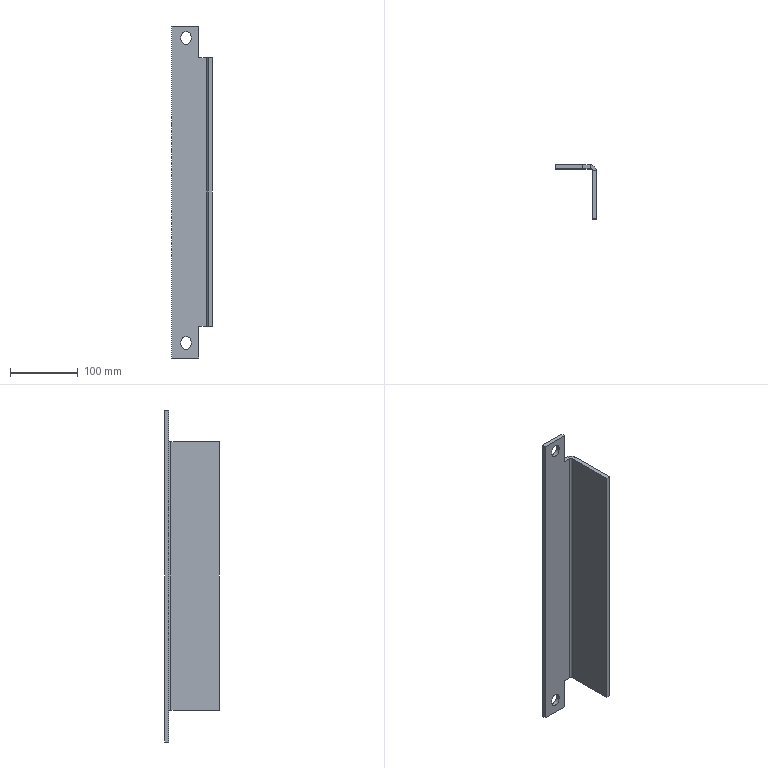Part | SolidWorks | features ICE 2, FlatPattern 1, SMBaseFlange 1, SheetMetal 1 | 1 solid | 28 faces | box 60 x 80 x 490 mm | volume 331985 mm3 | plane 20 | cylinder 8 | commonest cylinder face diameters 15 x6 6 x1 18 x1
STEP:
#1=CARTESIAN_POINT('',(-38.8,-6.,-213.5));
#2=VERTEX_POINT('',#1);
#3=CARTESIAN_POINT('',(-31.3,-6.,-221.));
#4=VERTEX_POINT('',#3);
#5=CARTESIAN_POINT('',(-38.8,-6.,-221.));
#6=DIRECTION('',(0.,1.,0.));
#7=DIRECTION('',(-1.,0.,0.));
#8=AXIS2_PLACEMENT_3D('',#5,#6,#7);
#9=CIRCLE('',#8,7.5);
#10=EDGE_CURVE('',#2,#4,#9,.T.);
#11=ORIENTED_EDGE('',*,*,#10,.F.);
#12=CARTESIAN_POINT('',(-38.8,0.,-213.5));
#13=VERTEX_POINT('',#12);
#14=CARTESIAN_POINT('',(-38.8,-80.,-213.5));
#15=DIRECTION('',(0.,1.,0.));
#16=VECTOR('',#15,1000.);
#17=LINE('',#14,#16);
#18=EDGE_CURVE('',#2,#13,#17,.T.);
#19=ORIENTED_EDGE('',*,*,#18,.T.);
#20=CARTESIAN_POINT('',(-31.3,0.,-221.));
#21=VERTEX_POINT('',#20);
#22=CARTESIAN_POINT('',(-38.8,0.,-221.));
#23=DIRECTION('',(0.,1.,0.));
#24=DIRECTION('',(0.,0.,1.));
#25=AXIS2_PLACEMENT_3D('',#22,#23,#24);
#26=CIRCLE('',#25,7.5);
#27=EDGE_CURVE('',#13,#21,#26,.T.);
#28=ORIENTED_EDGE('',*,*,#27,.T.);
#29=CARTESIAN_POINT('',(-31.3,-80.,-221.));
#30=DIRECTION('',(0.,1.,0.));
#31=VECTOR('',#30,1000.);
#32=LINE('',#29,#31);
#33=EDGE_CURVE('',#4,#21,#32,.T.);
#34=ORIENTED_EDGE('',*,*,#33,.F.);
#35=EDGE_LOOP('',(#11,#19,#28,#34));
#36=FACE_OUTER_BOUND('',#35,.T.);
#37=CARTESIAN_POINT('',(-38.8,-80.,-221.));
#38=DIRECTION('',(0.,1.,0.));
#39=DIRECTION('',(0.,0.,1.));
#40=AXIS2_PLACEMENT_3D('',#37,#38,#39);
#41=CYLINDRICAL_SURFACE('',#40,7.5);
#42=ADVANCED_FACE('',(#36),#41,.F.);
#43=CARTESIAN_POINT('',(-38.8,-6.,236.5));
#44=VERTEX_POINT('',#43);
#45=CARTESIAN_POINT('',(-31.3,-6.,229.));
#46=VERTEX_POINT('',#45);
#47=CARTESIAN_POINT('',(-38.8,-6.,229.));
#48=DIRECTION('',(0.,1.,0.));
#49=DIRECTION('',(-1.,0.,0.));
#50=AXIS2_PLACEMENT_3D('',#47,#48,#49);
#51=CIRCLE('',#50,7.5);
#52=EDGE_CURVE('',#44,#46,#51,.T.);
#53=ORIENTED_EDGE('',*,*,#52,.F.);
#54=CARTESIAN_POINT('',(-38.8,0.,236.5));
#55=VERTEX_POINT('',#54);
#56=CARTESIAN_POINT('',(-38.8,-80.,236.5));
#57=DIRECTION('',(0.,1.,0.));
#58=VECTOR('',#57,1000.);
#59=LINE('',#56,#58);
#60=EDGE_CURVE('',#44,#55,#59,.T.);
#61=ORIENTED_EDGE('',*,*,#60,.T.);
#62=CARTESIAN_POINT('',(-31.3,0.,229.));
#63=VERTEX_POINT('',#62);
#64=CARTESIAN_POINT('',(-38.8,0.,229.));
#65=DIRECTION('',(0.,1.,0.));
#66=DIRECTION('',(0.,0.,1.));
#67=AXIS2_PLACEMENT_3D('',#64,#65,#66);
#68=CIRCLE('',#67,7.5);
#69=EDGE_CURVE('',#55,#63,#68,.T.);
#70=ORIENTED_EDGE('',*,*,#69,.T.);
#71=CARTESIAN_POINT('',(-31.3,-80.,229.));
#72=DIRECTION('',(0.,1.,0.));
#73=VECTOR('',#72,1000.);
#74=LINE('',#71,#73);
#75=EDGE_CURVE('',#46,#63,#74,.T.);
#76=ORIENTED_EDGE('',*,*,#75,.F.);
#77=EDGE_LOOP('',(#53,#61,#70,#76));
#78=FACE_OUTER_BOUND('',#77,.T.);
#79=CARTESIAN_POINT('',(-38.8,-80.,229.));
#80=DIRECTION('',(0.,1.,0.));
#81=DIRECTION('',(0.,0.,1.));
#82=AXIS2_PLACEMENT_3D('',#79,#80,#81);
#83=CYLINDRICAL_SURFACE('',#82,7.5);
#84=ADVANCED_FACE('',(#78),#83,.F.);
#85=CARTESIAN_POINT('',(-6.,-9.,-198.));
#86=VERTEX_POINT('',#85);
#87=CARTESIAN_POINT('',(-6.,-80.,-198.));
#88=VERTEX_POINT('',#87);
#89=CARTESIAN_POINT('',(-6.,0.,-198.));
#90=DIRECTION('',(0.,-1.,0.));
#91=VECTOR('',#90,1000.);
#92=LINE('',#89,#91);
#93=EDGE_CURVE('',#86,#88,#92,.T.);
#94=ORIENTED_EDGE('',*,*,#93,.F.);
#95=CARTESIAN_POINT('',(0.,-9.,-198.));
#96=VERTEX_POINT('',#95);
#97=CARTESIAN_POINT('',(-6.,-9.,-198.));
#98=DIRECTION('',(1.,0.,0.));
#99=VECTOR('',#98,1000.);
#100=LINE('',#97,#99);
#101=EDGE_CURVE('',#86,#96,#100,.T.);
#102=ORIENTED_EDGE('',*,*,#101,.T.);
#103=CARTESIAN_POINT('',(0.,-80.,-198.));
#104=VERTEX_POINT('',#103);
#105=CARTESIAN_POINT('',(0.,-80.,-198.));
#106=DIRECTION('',(0.,-1.,0.));
#107=VECTOR('',#106,1000.);
#108=LINE('',#105,#107);
#109=EDGE_CURVE('',#96,#104,#108,.T.);
#110=ORIENTED_EDGE('',*,*,#109,.T.);
#111=CARTESIAN_POINT('',(-20.,-80.,-198.));
#112=DIRECTION('',(1.,0.,0.));
#113=VECTOR('',#112,1000.);
#114=LINE('',#111,#113);
#115=EDGE_CURVE('',#88,#104,#114,.T.);
#116=ORIENTED_EDGE('',*,*,#115,.F.);
#117=EDGE_LOOP('',(#94,#102,#110,#116));
#118=FACE_OUTER_BOUND('',#117,.T.);
#119=CARTESIAN_POINT('',(-20.,-80.,-198.));
#120=DIRECTION('',(0.,0.,1.));
#121=DIRECTION('',(1.,0.,0.));
#122=AXIS2_PLACEMENT_3D('',#119,#120,#121);
#123=PLANE('',#122);
#124=ADVANCED_FACE('',(#118),#123,.F.);
#125=CARTESIAN_POINT('',(-20.,0.,-198.));
#126=VERTEX_POINT('',#125);
#127=CARTESIAN_POINT('',(-9.,0.,-198.));
#128=VERTEX_POINT('',#127);
#129=CARTESIAN_POINT('',(-20.,0.,-198.));
#130=DIRECTION('',(1.,0.,0.));
#131=VECTOR('',#130,1000.);
#132=LINE('',#129,#131);
#133=EDGE_CURVE('',#126,#128,#132,.T.);
#134=ORIENTED_EDGE('',*,*,#133,.T.);
#135=CARTESIAN_POINT('',(-9.,-6.,-198.));
#136=VERTEX_POINT('',#135);
#137=CARTESIAN_POINT('',(-9.,0.,-198.));
#138=DIRECTION('',(0.,-1.,0.));
#139=VECTOR('',#138,1000.);
#140=LINE('',#137,#139);
#141=EDGE_CURVE('',#128,#136,#140,.T.);
#142=ORIENTED_EDGE('',*,*,#141,.T.);
#143=CARTESIAN_POINT('',(-20.,-6.,-198.));
#144=VERTEX_POINT('',#143);
#145=CARTESIAN_POINT('',(0.,-6.,-198.));
#146=DIRECTION('',(1.,0.,0.));
#147=VECTOR('',#146,1000.);
#148=LINE('',#145,#147);
#149=EDGE_CURVE('',#144,#136,#148,.T.);
#150=ORIENTED_EDGE('',*,*,#149,.F.);
#151=CARTESIAN_POINT('',(-20.,-80.,-198.));
#152=DIRECTION('',(0.,-1.,0.));
#153=VECTOR('',#152,1000.);
#154=LINE('',#151,#153);
#155=EDGE_CURVE('',#126,#144,#154,.T.);
#156=ORIENTED_EDGE('',*,*,#155,.F.);
#157=EDGE_LOOP('',(#134,#142,#150,#156));
#158=FACE_OUTER_BOUND('',#157,.T.);
#159=CARTESIAN_POINT('',(-20.,-80.,-198.));
#160=DIRECTION('',(0.,0.,1.));
#161=DIRECTION('',(1.,0.,0.));
#162=AXIS2_PLACEMENT_3D('',#159,#160,#161);
#163=PLANE('',#162);
#164=ADVANCED_FACE('',(#158),#163,.F.);
#165=CARTESIAN_POINT('',(-9.,-6.,198.));
#166=VERTEX_POINT('',#165);
#167=CARTESIAN_POINT('',(-20.,-6.,198.));
#168=VERTEX_POINT('',#167);
#169=CARTESIAN_POINT('',(0.,-6.,198.));
#170=DIRECTION('',(-1.,0.,0.));
#171=VECTOR('',#170,1000.);
#172=LINE('',#169,#171);
#173=EDGE_CURVE('',#166,#168,#172,.T.);
#174=ORIENTED_EDGE('',*,*,#173,.F.);
#175=CARTESIAN_POINT('',(-9.,0.,198.));
#176=VERTEX_POINT('',#175);
#177=CARTESIAN_POINT('',(-9.,-6.,198.));
#178=DIRECTION('',(0.,1.,0.));
#179=VECTOR('',#178,1000.);
#180=LINE('',#177,#179);
#181=EDGE_CURVE('',#166,#176,#180,.T.);
#182=ORIENTED_EDGE('',*,*,#181,.T.);
#183=CARTESIAN_POINT('',(-20.,0.,198.));
#184=VERTEX_POINT('',#183);
#185=CARTESIAN_POINT('',(-20.,0.,198.));
#186=DIRECTION('',(1.,0.,0.));
#187=VECTOR('',#186,1000.);
#188=LINE('',#185,#187);
#189=EDGE_CURVE('',#184,#176,#188,.T.);
#190=ORIENTED_EDGE('',*,*,#189,.F.);
#191=CARTESIAN_POINT('',(-20.,-80.,198.));
#192=DIRECTION('',(0.,1.,0.));
#193=VECTOR('',#192,1000.);
#194=LINE('',#191,#193);
#195=EDGE_CURVE('',#168,#184,#194,.T.);
#196=ORIENTED_EDGE('',*,*,#195,.F.);
#197=EDGE_LOOP('',(#174,#182,#190,#196));
#198=FACE_OUTER_BOUND('',#197,.T.);
#199=CARTESIAN_POINT('',(-20.,-80.,198.));
#200=DIRECTION('',(0.,0.,-1.));
#201=DIRECTION('',(-1.,0.,0.));
#202=AXIS2_PLACEMENT_3D('',#199,#200,#201);
#203=PLANE('',#202);
#204=ADVANCED_FACE('',(#198),#203,.F.);
#205=CARTESIAN_POINT('',(0.,-80.,198.));
#206=VERTEX_POINT('',#205);
#207=CARTESIAN_POINT('',(0.,-9.,198.));
#208=VERTEX_POINT('',#207);
#209=CARTESIAN_POINT('',(0.,-80.,198.));
#210=DIRECTION('',(0.,1.,0.));
#211=VECTOR('',#210,1000.);
#212=LINE('',#209,#211);
#213=EDGE_CURVE('',#206,#208,#212,.T.);
#214=ORIENTED_EDGE('',*,*,#213,.T.);
#215=CARTESIAN_POINT('',(-6.,-9.,198.));
#216=VERTEX_POINT('',#215);
#217=CARTESIAN_POINT('',(0.,-9.,198.));
#218=DIRECTION('',(-1.,0.,0.));
#219=VECTOR('',#218,1000.);
#220=LINE('',#217,#219);
#221=EDGE_CURVE('',#208,#216,#220,.T.);
#222=ORIENTED_EDGE('',*,*,#221,.T.);
#223=CARTESIAN_POINT('',(-6.,-80.,198.));
#224=VERTEX_POINT('',#223);
#225=CARTESIAN_POINT('',(-6.,0.,198.));
#226=DIRECTION('',(0.,1.,0.));
#227=VECTOR('',#226,1000.);
#228=LINE('',#225,#227);
#229=EDGE_CURVE('',#224,#216,#228,.T.);
#230=ORIENTED_EDGE('',*,*,#229,.F.);
#231=CARTESIAN_POINT('',(-20.,-80.,198.));
#232=DIRECTION('',(1.,0.,0.));
#233=VECTOR('',#232,1000.);
#234=LINE('',#231,#233);
#235=EDGE_CURVE('',#224,#206,#234,.T.);
#236=ORIENTED_EDGE('',*,*,#235,.T.);
#237=EDGE_LOOP('',(#214,#222,#230,#236));
#238=FACE_OUTER_BOUND('',#237,.T.);
#239=CARTESIAN_POINT('',(-20.,-80.,198.));
#240=DIRECTION('',(0.,0.,-1.));
#241=DIRECTION('',(-1.,0.,0.));
#242=AXIS2_PLACEMENT_3D('',#239,#240,#241);
#243=PLANE('',#242);
#244=ADVANCED_FACE('',(#238),#243,.F.);
#245=CARTESIAN_POINT('',(-20.,-6.,-245.));
#246=VERTEX_POINT('',#245);
#247=CARTESIAN_POINT('',(-20.,0.,-245.));
#248=VERTEX_POINT('',#247);
#249=CARTESIAN_POINT('',(-20.,-80.,-245.));
#250=DIRECTION('',(0.,1.,0.));
#251=VECTOR('',#250,1000.);
#252=LINE('',#249,#251);
#253=EDGE_CURVE('',#246,#248,#252,.T.);
#254=ORIENTED_EDGE('',*,*,#253,.F.);
#255=CARTESIAN_POINT('',(-60.,-6.,-245.));
#256=VERTEX_POINT('',#255);
#257=CARTESIAN_POINT('',(0.,-6.,-245.));
#258=DIRECTION('',(1.,0.,0.));
#259=VECTOR('',#258,1000.);
#260=LINE('',#257,#259);
#261=EDGE_CURVE('',#256,#246,#260,.T.);
#262=ORIENTED_EDGE('',*,*,#261,.F.);
#263=CARTESIAN_POINT('',(-60.,0.,-245.));
#264=VERTEX_POINT('',#263);
#265=CARTESIAN_POINT('',(-60.,-6.,-245.));
#266=DIRECTION('',(0.,1.,0.));
#267=VECTOR('',#266,1000.);
#268=LINE('',#265,#267);
#269=EDGE_CURVE('',#256,#264,#268,.T.);
#270=ORIENTED_EDGE('',*,*,#269,.T.);
#271=CARTESIAN_POINT('',(0.,0.,-245.));
#272=DIRECTION('',(1.,0.,0.));
#273=VECTOR('',#272,1000.);
#274=LINE('',#271,#273);
#275=EDGE_CURVE('',#264,#248,#274,.T.);
#276=ORIENTED_EDGE('',*,*,#275,.T.);
#277=EDGE_LOOP('',(#254,#262,#270,#276));
#278=FACE_OUTER_BOUND('',#277,.T.);
#279=CARTESIAN_POINT('',(-6.,-9.,-245.));
#280=DIRECTION('',(0.,0.,-1.));
#281=DIRECTION('',(-1.,0.,0.));
#282=AXIS2_PLACEMENT_3D('',#279,#280,#281);
#283=PLANE('',#282);
#284=ADVANCED_FACE('',(#278),#283,.T.);
#285=CARTESIAN_POINT('',(-6.,-80.,245.));
#286=DIRECTION('',(0.,0.,-1.));
#287=VECTOR('',#286,1000.);
#288=LINE('',#285,#287);
#289=EDGE_CURVE('',#224,#88,#288,.T.);
#290=ORIENTED_EDGE('',*,*,#289,.F.);
#291=ORIENTED_EDGE('',*,*,#229,.T.);
#292=CARTESIAN_POINT('',(-6.,-9.,245.));
#293=DIRECTION('',(0.,0.,-1.));
#294=VECTOR('',#293,1000.);
#295=LINE('',#292,#294);
#296=EDGE_CURVE('',#216,#86,#295,.T.);
#297=ORIENTED_EDGE('',*,*,#296,.T.);
#298=ORIENTED_EDGE('',*,*,#93,.T.);
#299=EDGE_LOOP('',(#290,#291,#297,#298));
#300=FACE_OUTER_BOUND('',#299,.T.);
#301=CARTESIAN_POINT('',(-6.,0.,245.));
#302=DIRECTION('',(1.,0.,0.));
#303=DIRECTION('',(0.,1.,0.));
#304=AXIS2_PLACEMENT_3D('',#301,#302,#303);
#305=PLANE('',#304);
#306=ADVANCED_FACE('',(#300),#305,.F.);
#307=ORIENTED_EDGE('',*,*,#235,.F.);
#308=ORIENTED_EDGE('',*,*,#289,.T.);
#309=ORIENTED_EDGE('',*,*,#115,.T.);
#310=CARTESIAN_POINT('',(0.,-80.,245.));
#311=DIRECTION('',(0.,0.,-1.));
#312=VECTOR('',#311,1000.);
#313=LINE('',#310,#312);
#314=EDGE_CURVE('',#206,#104,#313,.T.);
#315=ORIENTED_EDGE('',*,*,#314,.F.);
#316=EDGE_LOOP('',(#307,#308,#309,#315));
#317=FACE_OUTER_BOUND('',#316,.T.);
#318=CARTESIAN_POINT('',(0.,-80.,245.));
#319=DIRECTION('',(0.,-1.,0.));
#320=DIRECTION('',(0.,0.,-1.));
#321=AXIS2_PLACEMENT_3D('',#318,#319,#320);
#322=PLANE('',#321);
#323=ADVANCED_FACE('',(#317),#322,.T.);
#324=ORIENTED_EDGE('',*,*,#213,.F.);
#325=ORIENTED_EDGE('',*,*,#314,.T.);
#326=ORIENTED_EDGE('',*,*,#109,.F.);
#327=CARTESIAN_POINT('',(0.,-9.,245.));
#328=DIRECTION('',(0.,0.,-1.));
#329=VECTOR('',#328,1000.);
#330=LINE('',#327,#329);
#331=EDGE_CURVE('',#208,#96,#330,.T.);
#332=ORIENTED_EDGE('',*,*,#331,.F.);
#333=EDGE_LOOP('',(#324,#325,#326,#332));
#334=FACE_OUTER_BOUND('',#333,.T.);
#335=CARTESIAN_POINT('',(0.,0.,245.));
#336=DIRECTION('',(1.,0.,0.));
#337=DIRECTION('',(0.,1.,0.));
#338=AXIS2_PLACEMENT_3D('',#335,#336,#337);
#339=PLANE('',#338);
#340=ADVANCED_FACE('',(#334),#339,.T.);
#341=CARTESIAN_POINT('',(-9.,-9.,198.));
#342=DIRECTION('',(0.,0.,1.));
#343=DIRECTION('',(-1.,0.,0.));
#344=AXIS2_PLACEMENT_3D('',#341,#342,#343);
#345=CIRCLE('',#344,9.);
#346=EDGE_CURVE('',#208,#176,#345,.T.);
#347=ORIENTED_EDGE('',*,*,#346,.F.);
#348=ORIENTED_EDGE('',*,*,#331,.T.);
#349=CARTESIAN_POINT('',(-9.,-9.,-198.));
#350=DIRECTION('',(0.,0.,-1.));
#351=DIRECTION('',(1.,0.,0.));
#352=AXIS2_PLACEMENT_3D('',#349,#350,#351);
#353=CIRCLE('',#352,9.);
#354=EDGE_CURVE('',#128,#96,#353,.T.);
#355=ORIENTED_EDGE('',*,*,#354,.F.);
#356=CARTESIAN_POINT('',(-9.,0.,245.));
#357=DIRECTION('',(0.,0.,-1.));
#358=VECTOR('',#357,1000.);
#359=LINE('',#356,#358);
#360=EDGE_CURVE('',#176,#128,#359,.T.);
#361=ORIENTED_EDGE('',*,*,#360,.F.);
#362=EDGE_LOOP('',(#347,#348,#355,#361));
#363=FACE_OUTER_BOUND('',#362,.T.);
#364=CARTESIAN_POINT('',(-9.,-9.,245.));
#365=DIRECTION('',(0.,0.,-1.));
#366=DIRECTION('',(-1.,0.,0.));
#367=AXIS2_PLACEMENT_3D('',#364,#365,#366);
#368=CYLINDRICAL_SURFACE('',#367,9.);
#369=ADVANCED_FACE('',(#363),#368,.T.);
#370=ORIENTED_EDGE('',*,*,#189,.T.);
#371=ORIENTED_EDGE('',*,*,#360,.T.);
#372=ORIENTED_EDGE('',*,*,#133,.F.);
#373=CARTESIAN_POINT('',(-20.,0.,-245.));
#374=DIRECTION('',(0.,0.,1.));
#375=VECTOR('',#374,1000.);
#376=LINE('',#373,#375);
#377=EDGE_CURVE('',#248,#126,#376,.T.);
#378=ORIENTED_EDGE('',*,*,#377,.F.);
#379=ORIENTED_EDGE('',*,*,#275,.F.);
#380=CARTESIAN_POINT('',(-60.,0.,245.));
#381=VERTEX_POINT('',#380);
#382=CARTESIAN_POINT('',(-60.,0.,245.));
#383=DIRECTION('',(0.,0.,-1.));
#384=VECTOR('',#383,1000.);
#385=LINE('',#382,#384);
#386=EDGE_CURVE('',#381,#264,#385,.T.);
#387=ORIENTED_EDGE('',*,*,#386,.F.);
#388=CARTESIAN_POINT('',(-20.,0.,245.));
#389=VERTEX_POINT('',#388);
#390=CARTESIAN_POINT('',(0.,0.,245.));
#391=DIRECTION('',(1.,0.,0.));
#392=VECTOR('',#391,1000.);
#393=LINE('',#390,#392);
#394=EDGE_CURVE('',#381,#389,#393,.T.);
#395=ORIENTED_EDGE('',*,*,#394,.T.);
#396=CARTESIAN_POINT('',(-20.,0.,245.));
#397=DIRECTION('',(0.,0.,1.));
#398=VECTOR('',#397,1000.);
#399=LINE('',#396,#398);
#400=EDGE_CURVE('',#184,#389,#399,.T.);
#401=ORIENTED_EDGE('',*,*,#400,.F.);
#402=EDGE_LOOP('',(#370,#371,#372,#378,#379,#387,#395,#401));
#403=FACE_OUTER_BOUND('',#402,.T.);
#404=CARTESIAN_POINT('',(-31.3,0.,-225.));
#405=VERTEX_POINT('',#404);
#406=CARTESIAN_POINT('',(-46.3,0.,-225.));
#407=VERTEX_POINT('',#406);
#408=CARTESIAN_POINT('',(-38.8,0.,-225.));
#409=DIRECTION('',(0.,1.,0.));
#410=DIRECTION('',(0.,0.,1.));
#411=AXIS2_PLACEMENT_3D('',#408,#409,#410);
#412=CIRCLE('',#411,7.5);
#413=EDGE_CURVE('',#405,#407,#412,.T.);
#414=ORIENTED_EDGE('',*,*,#413,.F.);
#415=CARTESIAN_POINT('',(-31.3,0.,-225.));
#416=DIRECTION('',(0.,0.,-1.));
#417=VECTOR('',#416,1000.);
#418=LINE('',#415,#417);
#419=EDGE_CURVE('',#21,#405,#418,.T.);
#420=ORIENTED_EDGE('',*,*,#419,.F.);
#421=ORIENTED_EDGE('',*,*,#27,.F.);
#422=CARTESIAN_POINT('',(-46.3,0.,-221.));
#423=VERTEX_POINT('',#422);
#424=CARTESIAN_POINT('',(-38.8,0.,-221.));
#425=DIRECTION('',(0.,1.,0.));
#426=DIRECTION('',(0.,0.,1.));
#427=AXIS2_PLACEMENT_3D('',#424,#425,#426);
#428=CIRCLE('',#427,7.5);
#429=EDGE_CURVE('',#423,#13,#428,.T.);
#430=ORIENTED_EDGE('',*,*,#429,.F.);
#431=CARTESIAN_POINT('',(-46.3,0.,-225.));
#432=DIRECTION('',(0.,0.,1.));
#433=VECTOR('',#432,1000.);
#434=LINE('',#431,#433);
#435=EDGE_CURVE('',#407,#423,#434,.T.);
#436=ORIENTED_EDGE('',*,*,#435,.F.);
#437=EDGE_LOOP('',(#414,#420,#421,#430,#436));
#438=FACE_BOUND('',#437,.T.);
#439=CARTESIAN_POINT('',(-31.3,0.,225.));
#440=VERTEX_POINT('',#439);
#441=CARTESIAN_POINT('',(-46.3,0.,225.));
#442=VERTEX_POINT('',#441);
#443=CARTESIAN_POINT('',(-38.8,0.,225.));
#444=DIRECTION('',(0.,1.,0.));
#445=DIRECTION('',(0.,0.,1.));
#446=AXIS2_PLACEMENT_3D('',#443,#444,#445);
#447=CIRCLE('',#446,7.5);
#448=EDGE_CURVE('',#440,#442,#447,.T.);
#449=ORIENTED_EDGE('',*,*,#448,.F.);
#450=CARTESIAN_POINT('',(-31.3,0.,225.));
#451=DIRECTION('',(0.,0.,-1.));
#452=VECTOR('',#451,1000.);
#453=LINE('',#450,#452);
#454=EDGE_CURVE('',#63,#440,#453,.T.);
#455=ORIENTED_EDGE('',*,*,#454,.F.);
#456=ORIENTED_EDGE('',*,*,#69,.F.);
#457=CARTESIAN_POINT('',(-46.3,0.,229.));
#458=VERTEX_POINT('',#457);
#459=CARTESIAN_POINT('',(-38.8,0.,229.));
#460=DIRECTION('',(0.,1.,0.));
#461=DIRECTION('',(0.,0.,1.));
#462=AXIS2_PLACEMENT_3D('',#459,#460,#461);
#463=CIRCLE('',#462,7.5);
#464=EDGE_CURVE('',#458,#55,#463,.T.);
#465=ORIENTED_EDGE('',*,*,#464,.F.);
#466=CARTESIAN_POINT('',(-46.3,0.,225.));
#467=DIRECTION('',(0.,0.,1.));
#468=VECTOR('',#467,1000.);
#469=LINE('',#466,#468);
#470=EDGE_CURVE('',#442,#458,#469,.T.);
#471=ORIENTED_EDGE('',*,*,#470,.F.);
#472=EDGE_LOOP('',(#449,#455,#456,#465,#471));
#473=FACE_BOUND('',#472,.T.);
#474=CARTESIAN_POINT('',(0.,0.,245.));
#475=DIRECTION('',(0.,1.,0.));
#476=DIRECTION('',(-1.,0.,0.));
#477=AXIS2_PLACEMENT_3D('',#474,#475,#476);
#478=PLANE('',#477);
#479=ADVANCED_FACE('',(#403,#438,#473),#478,.T.);
#480=ORIENTED_EDGE('',*,*,#269,.F.);
#481=CARTESIAN_POINT('',(-60.,-6.,245.));
#482=VERTEX_POINT('',#481);
#483=CARTESIAN_POINT('',(-60.,-6.,245.));
#484=DIRECTION('',(0.,0.,-1.));
#485=VECTOR('',#484,1000.);
#486=LINE('',#483,#485);
#487=EDGE_CURVE('',#482,#256,#486,.T.);
#488=ORIENTED_EDGE('',*,*,#487,.F.);
#489=CARTESIAN_POINT('',(-60.,-6.,245.));
#490=DIRECTION('',(0.,1.,0.));
#491=VECTOR('',#490,1000.);
#492=LINE('',#489,#491);
#493=EDGE_CURVE('',#482,#381,#492,.T.);
#494=ORIENTED_EDGE('',*,*,#493,.T.);
#495=ORIENTED_EDGE('',*,*,#386,.T.);
#496=EDGE_LOOP('',(#480,#488,#494,#495));
#497=FACE_OUTER_BOUND('',#496,.T.);
#498=CARTESIAN_POINT('',(-60.,-6.,245.));
#499=DIRECTION('',(-1.,0.,0.));
#500=DIRECTION('',(0.,0.,1.));
#501=AXIS2_PLACEMENT_3D('',#498,#499,#500);
#502=PLANE('',#501);
#503=ADVANCED_FACE('',(#497),#502,.T.);
#504=CARTESIAN_POINT('',(-31.3,-6.,-225.));
#505=VERTEX_POINT('',#504);
#506=CARTESIAN_POINT('',(-31.3,-6.,245.));
#507=DIRECTION('',(0.,0.,-1.));
#508=VECTOR('',#507,1000.);
#509=LINE('',#506,#508);
#510=EDGE_CURVE('',#4,#505,#509,.T.);
#511=ORIENTED_EDGE('',*,*,#510,.T.);
#512=CARTESIAN_POINT('',(-46.3,-6.,-225.));
#513=VERTEX_POINT('',#512);
#514=CARTESIAN_POINT('',(-38.8,-6.,-225.));
#515=DIRECTION('',(0.,1.,0.));
#516=DIRECTION('',(-1.,0.,0.));
#517=AXIS2_PLACEMENT_3D('',#514,#515,#516);
#518=CIRCLE('',#517,7.5);
#519=EDGE_CURVE('',#505,#513,#518,.T.);
#520=ORIENTED_EDGE('',*,*,#519,.T.);
#521=CARTESIAN_POINT('',(-46.3,-6.,-221.));
#522=VERTEX_POINT('',#521);
#523=CARTESIAN_POINT('',(-46.3,-6.,245.));
#524=DIRECTION('',(0.,0.,1.));
#525=VECTOR('',#524,1000.);
#526=LINE('',#523,#525);
#527=EDGE_CURVE('',#513,#522,#526,.T.);
#528=ORIENTED_EDGE('',*,*,#527,.T.);
#529=CARTESIAN_POINT('',(-38.8,-6.,-221.));
#530=DIRECTION('',(0.,1.,0.));
#531=DIRECTION('',(-1.,0.,0.));
#532=AXIS2_PLACEMENT_3D('',#529,#530,#531);
#533=CIRCLE('',#532,7.5);
#534=EDGE_CURVE('',#522,#2,#533,.T.);
#535=ORIENTED_EDGE('',*,*,#534,.T.);
#536=ORIENTED_EDGE('',*,*,#10,.T.);
#537=EDGE_LOOP('',(#511,#520,#528,#535,#536));
#538=FACE_BOUND('',#537,.T.);
#539=CARTESIAN_POINT('',(-31.3,-6.,225.));
#540=VERTEX_POINT('',#539);
#541=CARTESIAN_POINT('',(-31.3,-6.,245.));
#542=DIRECTION('',(0.,0.,-1.));
#543=VECTOR('',#542,1000.);
#544=LINE('',#541,#543);
#545=EDGE_CURVE('',#46,#540,#544,.T.);
#546=ORIENTED_EDGE('',*,*,#545,.T.);
#547=CARTESIAN_POINT('',(-46.3,-6.,225.));
#548=VERTEX_POINT('',#547);
#549=CARTESIAN_POINT('',(-38.8,-6.,225.));
#550=DIRECTION('',(0.,1.,0.));
#551=DIRECTION('',(-1.,0.,0.));
#552=AXIS2_PLACEMENT_3D('',#549,#550,#551);
#553=CIRCLE('',#552,7.5);
#554=EDGE_CURVE('',#540,#548,#553,.T.);
#555=ORIENTED_EDGE('',*,*,#554,.T.);
#556=CARTESIAN_POINT('',(-46.3,-6.,229.));
#557=VERTEX_POINT('',#556);
#558=CARTESIAN_POINT('',(-46.3,-6.,245.));
#559=DIRECTION('',(0.,0.,1.));
#560=VECTOR('',#559,1000.);
#561=LINE('',#558,#560);
#562=EDGE_CURVE('',#548,#557,#561,.T.);
#563=ORIENTED_EDGE('',*,*,#562,.T.);
#564=CARTESIAN_POINT('',(-38.8,-6.,229.));
#565=DIRECTION('',(0.,1.,0.));
#566=DIRECTION('',(-1.,0.,0.));
#567=AXIS2_PLACEMENT_3D('',#564,#565,#566);
#568=CIRCLE('',#567,7.5);
#569=EDGE_CURVE('',#557,#44,#568,.T.);
#570=ORIENTED_EDGE('',*,*,#569,.T.);
#571=ORIENTED_EDGE('',*,*,#52,.T.);
#572=EDGE_LOOP('',(#546,#555,#563,#570,#571));
#573=FACE_BOUND('',#572,.T.);
#574=CARTESIAN_POINT('',(-9.,-6.,245.));
#575=DIRECTION('',(0.,0.,-1.));
#576=VECTOR('',#575,1000.);
#577=LINE('',#574,#576);
#578=EDGE_CURVE('',#166,#136,#577,.T.);
#579=ORIENTED_EDGE('',*,*,#578,.F.);
#580=ORIENTED_EDGE('',*,*,#173,.T.);
#581=CARTESIAN_POINT('',(-20.,-6.,245.));
#582=VERTEX_POINT('',#581);
#583=CARTESIAN_POINT('',(-20.,-6.,245.));
#584=DIRECTION('',(0.,0.,1.));
#585=VECTOR('',#584,1000.);
#586=LINE('',#583,#585);
#587=EDGE_CURVE('',#168,#582,#586,.T.);
#588=ORIENTED_EDGE('',*,*,#587,.T.);
#589=CARTESIAN_POINT('',(0.,-6.,245.));
#590=DIRECTION('',(1.,0.,0.));
#591=VECTOR('',#590,1000.);
#592=LINE('',#589,#591);
#593=EDGE_CURVE('',#482,#582,#592,.T.);
#594=ORIENTED_EDGE('',*,*,#593,.F.);
#595=ORIENTED_EDGE('',*,*,#487,.T.);
#596=ORIENTED_EDGE('',*,*,#261,.T.);
#597=CARTESIAN_POINT('',(-20.,-6.,245.));
#598=DIRECTION('',(0.,0.,1.));
#599=VECTOR('',#598,1000.);
#600=LINE('',#597,#599);
#601=EDGE_CURVE('',#246,#144,#600,.T.);
#602=ORIENTED_EDGE('',*,*,#601,.T.);
#603=ORIENTED_EDGE('',*,*,#149,.T.);
#604=EDGE_LOOP('',(#579,#580,#588,#594,#595,#596,#602,#603));
#605=FACE_OUTER_BOUND('',#604,.T.);
#606=CARTESIAN_POINT('',(0.,-6.,245.));
#607=DIRECTION('',(0.,1.,0.));
#608=DIRECTION('',(-1.,0.,0.));
#609=AXIS2_PLACEMENT_3D('',#606,#607,#608);
#610=PLANE('',#609);
#611=ADVANCED_FACE('',(#538,#573,#605),#610,.F.);
#612=ORIENTED_EDGE('',*,*,#296,.F.);
#613=CARTESIAN_POINT('',(-9.,-9.,198.));
#614=DIRECTION('',(0.,0.,1.));
#615=DIRECTION('',(-1.,0.,0.));
#616=AXIS2_PLACEMENT_3D('',#613,#614,#615);
#617=CIRCLE('',#616,3.);
#618=EDGE_CURVE('',#216,#166,#617,.T.);
#619=ORIENTED_EDGE('',*,*,#618,.T.);
#620=ORIENTED_EDGE('',*,*,#578,.T.);
#621=CARTESIAN_POINT('',(-9.,-9.,-198.));
#622=DIRECTION('',(0.,0.,-1.));
#623=DIRECTION('',(1.,0.,0.));
#624=AXIS2_PLACEMENT_3D('',#621,#622,#623);
#625=CIRCLE('',#624,3.);
#626=EDGE_CURVE('',#136,#86,#625,.T.);
#627=ORIENTED_EDGE('',*,*,#626,.T.);
#628=EDGE_LOOP('',(#612,#619,#620,#627));
#629=FACE_OUTER_BOUND('',#628,.T.);
#630=CARTESIAN_POINT('',(-9.,-9.,245.));
#631=DIRECTION('',(0.,0.,-1.));
#632=DIRECTION('',(-1.,0.,0.));
#633=AXIS2_PLACEMENT_3D('',#630,#631,#632);
#634=CYLINDRICAL_SURFACE('',#633,3.);
#635=ADVANCED_FACE('',(#629),#634,.F.);
#636=CARTESIAN_POINT('',(-20.,-80.,245.));
#637=DIRECTION('',(0.,-1.,0.));
#638=VECTOR('',#637,1000.);
#639=LINE('',#636,#638);
#640=EDGE_CURVE('',#389,#582,#639,.T.);
#641=ORIENTED_EDGE('',*,*,#640,.F.);
#642=ORIENTED_EDGE('',*,*,#394,.F.);
#643=ORIENTED_EDGE('',*,*,#493,.F.);
#644=ORIENTED_EDGE('',*,*,#593,.T.);
#645=EDGE_LOOP('',(#641,#642,#643,#644));
#646=FACE_OUTER_BOUND('',#645,.T.);
#647=CARTESIAN_POINT('',(-9.,-9.,245.));
#648=DIRECTION('',(0.,0.,1.));
#649=DIRECTION('',(1.,0.,0.));
#650=AXIS2_PLACEMENT_3D('',#647,#648,#649);
#651=PLANE('',#650);
#652=ADVANCED_FACE('',(#646),#651,.T.);
#653=CARTESIAN_POINT('',(-31.3,-80.,225.));
#654=DIRECTION('',(0.,1.,0.));
#655=VECTOR('',#654,1000.);
#656=LINE('',#653,#655);
#657=EDGE_CURVE('',#540,#440,#656,.T.);
#658=ORIENTED_EDGE('',*,*,#657,.T.);
#659=ORIENTED_EDGE('',*,*,#448,.T.);
#660=CARTESIAN_POINT('',(-46.3,-80.,225.));
#661=DIRECTION('',(0.,1.,0.));
#662=VECTOR('',#661,1000.);
#663=LINE('',#660,#662);
#664=EDGE_CURVE('',#548,#442,#663,.T.);
#665=ORIENTED_EDGE('',*,*,#664,.F.);
#666=ORIENTED_EDGE('',*,*,#554,.F.);
#667=EDGE_LOOP('',(#658,#659,#665,#666));
#668=FACE_OUTER_BOUND('',#667,.T.);
#669=CARTESIAN_POINT('',(-38.8,-80.,225.));
#670=DIRECTION('',(0.,1.,0.));
#671=DIRECTION('',(0.,0.,1.));
#672=AXIS2_PLACEMENT_3D('',#669,#670,#671);
#673=CYLINDRICAL_SURFACE('',#672,7.5);
#674=ADVANCED_FACE('',(#668),#673,.F.);
#675=ORIENTED_EDGE('',*,*,#75,.T.);
#676=ORIENTED_EDGE('',*,*,#454,.T.);
#677=ORIENTED_EDGE('',*,*,#657,.F.);
#678=ORIENTED_EDGE('',*,*,#545,.F.);
#679=EDGE_LOOP('',(#675,#676,#677,#678));
#680=FACE_OUTER_BOUND('',#679,.T.);
#681=CARTESIAN_POINT('',(-31.3,-80.,225.));
#682=DIRECTION('',(1.,0.,0.));
#683=DIRECTION('',(0.,0.,-1.));
#684=AXIS2_PLACEMENT_3D('',#681,#682,#683);
#685=PLANE('',#684);
#686=ADVANCED_FACE('',(#680),#685,.F.);
#687=ORIENTED_EDGE('',*,*,#60,.F.);
#688=ORIENTED_EDGE('',*,*,#569,.F.);
#689=CARTESIAN_POINT('',(-46.3,-80.,229.));
#690=DIRECTION('',(0.,1.,0.));
#691=VECTOR('',#690,1000.);
#692=LINE('',#689,#691);
#693=EDGE_CURVE('',#557,#458,#692,.T.);
#694=ORIENTED_EDGE('',*,*,#693,.T.);
#695=ORIENTED_EDGE('',*,*,#464,.T.);
#696=EDGE_LOOP('',(#687,#688,#694,#695));
#697=FACE_OUTER_BOUND('',#696,.T.);
#698=CARTESIAN_POINT('',(-38.8,-80.,229.));
#699=DIRECTION('',(0.,1.,0.));
#700=DIRECTION('',(0.,0.,1.));
#701=AXIS2_PLACEMENT_3D('',#698,#699,#700);
#702=CYLINDRICAL_SURFACE('',#701,7.5);
#703=ADVANCED_FACE('',(#697),#702,.F.);
#704=ORIENTED_EDGE('',*,*,#664,.T.);
#705=ORIENTED_EDGE('',*,*,#470,.T.);
#706=ORIENTED_EDGE('',*,*,#693,.F.);
#707=ORIENTED_EDGE('',*,*,#562,.F.);
#708=EDGE_LOOP('',(#704,#705,#706,#707));
#709=FACE_OUTER_BOUND('',#708,.T.);
#710=CARTESIAN_POINT('',(-46.3,-80.,225.));
#711=DIRECTION('',(-1.,0.,0.));
#712=DIRECTION('',(0.,0.,1.));
#713=AXIS2_PLACEMENT_3D('',#710,#711,#712);
#714=PLANE('',#713);
#715=ADVANCED_FACE('',(#709),#714,.F.);
#716=CARTESIAN_POINT('',(-31.3,-80.,-225.));
#717=DIRECTION('',(0.,1.,0.));
#718=VECTOR('',#717,1000.);
#719=LINE('',#716,#718);
#720=EDGE_CURVE('',#505,#405,#719,.T.);
#721=ORIENTED_EDGE('',*,*,#720,.T.);
#722=ORIENTED_EDGE('',*,*,#413,.T.);
#723=CARTESIAN_POINT('',(-46.3,-80.,-225.));
#724=DIRECTION('',(0.,1.,0.));
#725=VECTOR('',#724,1000.);
#726=LINE('',#723,#725);
#727=EDGE_CURVE('',#513,#407,#726,.T.);
#728=ORIENTED_EDGE('',*,*,#727,.F.);
#729=ORIENTED_EDGE('',*,*,#519,.F.);
#730=EDGE_LOOP('',(#721,#722,#728,#729));
#731=FACE_OUTER_BOUND('',#730,.T.);
#732=CARTESIAN_POINT('',(-38.8,-80.,-225.));
#733=DIRECTION('',(0.,1.,0.));
#734=DIRECTION('',(0.,0.,1.));
#735=AXIS2_PLACEMENT_3D('',#732,#733,#734);
#736=CYLINDRICAL_SURFACE('',#735,7.5);
#737=ADVANCED_FACE('',(#731),#736,.F.);
#738=ORIENTED_EDGE('',*,*,#33,.T.);
#739=ORIENTED_EDGE('',*,*,#419,.T.);
#740=ORIENTED_EDGE('',*,*,#720,.F.);
#741=ORIENTED_EDGE('',*,*,#510,.F.);
#742=EDGE_LOOP('',(#738,#739,#740,#741));
#743=FACE_OUTER_BOUND('',#742,.T.);
#744=CARTESIAN_POINT('',(-31.3,-80.,-225.));
#745=DIRECTION('',(1.,0.,0.));
#746=DIRECTION('',(0.,0.,-1.));
#747=AXIS2_PLACEMENT_3D('',#744,#745,#746);
#748=PLANE('',#747);
#749=ADVANCED_FACE('',(#743),#748,.F.);
#750=ORIENTED_EDGE('',*,*,#18,.F.);
#751=ORIENTED_EDGE('',*,*,#534,.F.);
#752=CARTESIAN_POINT('',(-46.3,-80.,-221.));
#753=DIRECTION('',(0.,1.,0.));
#754=VECTOR('',#753,1000.);
#755=LINE('',#752,#754);
#756=EDGE_CURVE('',#522,#423,#755,.T.);
#757=ORIENTED_EDGE('',*,*,#756,.T.);
#758=ORIENTED_EDGE('',*,*,#429,.T.);
#759=EDGE_LOOP('',(#750,#751,#757,#758));
#760=FACE_OUTER_BOUND('',#759,.T.);
#761=CARTESIAN_POINT('',(-38.8,-80.,-221.));
#762=DIRECTION('',(0.,1.,0.));
#763=DIRECTION('',(0.,0.,1.));
#764=AXIS2_PLACEMENT_3D('',#761,#762,#763);
#765=CYLINDRICAL_SURFACE('',#764,7.5);
#766=ADVANCED_FACE('',(#760),#765,.F.);
#767=ORIENTED_EDGE('',*,*,#727,.T.);
#768=ORIENTED_EDGE('',*,*,#435,.T.);
#769=ORIENTED_EDGE('',*,*,#756,.F.);
#770=ORIENTED_EDGE('',*,*,#527,.F.);
#771=EDGE_LOOP('',(#767,#768,#769,#770));
#772=FACE_OUTER_BOUND('',#771,.T.);
#773=CARTESIAN_POINT('',(-46.3,-80.,-225.));
#774=DIRECTION('',(-1.,0.,0.));
#775=DIRECTION('',(0.,0.,1.));
#776=AXIS2_PLACEMENT_3D('',#773,#774,#775);
#777=PLANE('',#776);
#778=ADVANCED_FACE('',(#772),#777,.F.);
#779=ORIENTED_EDGE('',*,*,#181,.F.);
#780=ORIENTED_EDGE('',*,*,#618,.F.);
#781=ORIENTED_EDGE('',*,*,#221,.F.);
#782=ORIENTED_EDGE('',*,*,#346,.T.);
#783=EDGE_LOOP('',(#779,#780,#781,#782));
#784=FACE_OUTER_BOUND('',#783,.T.);
#785=CARTESIAN_POINT('',(-20.,-80.,198.));
#786=DIRECTION('',(0.,0.,-1.));
#787=DIRECTION('',(-1.,0.,0.));
#788=AXIS2_PLACEMENT_3D('',#785,#786,#787);
#789=PLANE('',#788);
#790=ADVANCED_FACE('',(#784),#789,.F.);
#791=ORIENTED_EDGE('',*,*,#195,.T.);
#792=ORIENTED_EDGE('',*,*,#400,.T.);
#793=ORIENTED_EDGE('',*,*,#640,.T.);
#794=ORIENTED_EDGE('',*,*,#587,.F.);
#795=EDGE_LOOP('',(#791,#792,#793,#794));
#796=FACE_OUTER_BOUND('',#795,.T.);
#797=CARTESIAN_POINT('',(-20.,0.,0.));
#798=DIRECTION('',(-1.,0.,0.));
#799=DIRECTION('',(0.,-1.,0.));
#800=AXIS2_PLACEMENT_3D('',#797,#798,#799);
#801=PLANE('',#800);
#802=ADVANCED_FACE('',(#796),#801,.F.);
#803=ORIENTED_EDGE('',*,*,#253,.T.);
#804=ORIENTED_EDGE('',*,*,#377,.T.);
#805=ORIENTED_EDGE('',*,*,#155,.T.);
#806=ORIENTED_EDGE('',*,*,#601,.F.);
#807=EDGE_LOOP('',(#803,#804,#805,#806));
#808=FACE_OUTER_BOUND('',#807,.T.);
#809=CARTESIAN_POINT('',(-20.,0.,0.));
#810=DIRECTION('',(-1.,0.,0.));
#811=DIRECTION('',(0.,-1.,0.));
#812=AXIS2_PLACEMENT_3D('',#809,#810,#811);
#813=PLANE('',#812);
#814=ADVANCED_FACE('',(#808),#813,.F.);
#815=ORIENTED_EDGE('',*,*,#101,.F.);
#816=ORIENTED_EDGE('',*,*,#626,.F.);
#817=ORIENTED_EDGE('',*,*,#141,.F.);
#818=ORIENTED_EDGE('',*,*,#354,.T.);
#819=EDGE_LOOP('',(#815,#816,#817,#818));
#820=FACE_OUTER_BOUND('',#819,.T.);
#821=CARTESIAN_POINT('',(-20.,-80.,-198.));
#822=DIRECTION('',(0.,0.,1.));
#823=DIRECTION('',(1.,0.,0.));
#824=AXIS2_PLACEMENT_3D('',#821,#822,#823);
#825=PLANE('',#824);
#826=ADVANCED_FACE('',(#820),#825,.F.);
#827=CLOSED_SHELL('',(#42,#84,#124,#164,#204,#244,#284,#306,#323,#340,#369,#479,#503,#611,#635,#652,#674,#686,#703,#715,#737,#749,#766,#778,#790,#802,#814,#826));
#828=MANIFOLD_SOLID_BREP('',#827);
#829=CARTESIAN_POINT('',(0.,0.,0.));
#830=DIRECTION('',(0.,0.,1.));
#831=DIRECTION('',(1.,0.,0.));
#832=AXIS2_PLACEMENT_3D('',#829,#830,#831);
#833=(LENGTH_UNIT()NAMED_UNIT(*)SI_UNIT(.MILLI.,.METRE.));
#834=UNCERTAINTY_MEASURE_WITH_UNIT(LENGTH_MEASURE(0.00001),#833,'','');
#835=(NAMED_UNIT(*)PLANE_ANGLE_UNIT()SI_UNIT($,.RADIAN.));
#836=(NAMED_UNIT(*)SI_UNIT($,.STERADIAN.)SOLID_ANGLE_UNIT());
#837=(GEOMETRIC_REPRESENTATION_CONTEXT(3)GLOBAL_UNCERTAINTY_ASSIGNED_CONTEXT((#834))GLOBAL_UNIT_ASSIGNED_CONTEXT((#833,#835,#836))REPRESENTATION_CONTEXT('',''));
#838=ADVANCED_BREP_SHAPE_REPRESENTATION('',(#828,#832),#837);